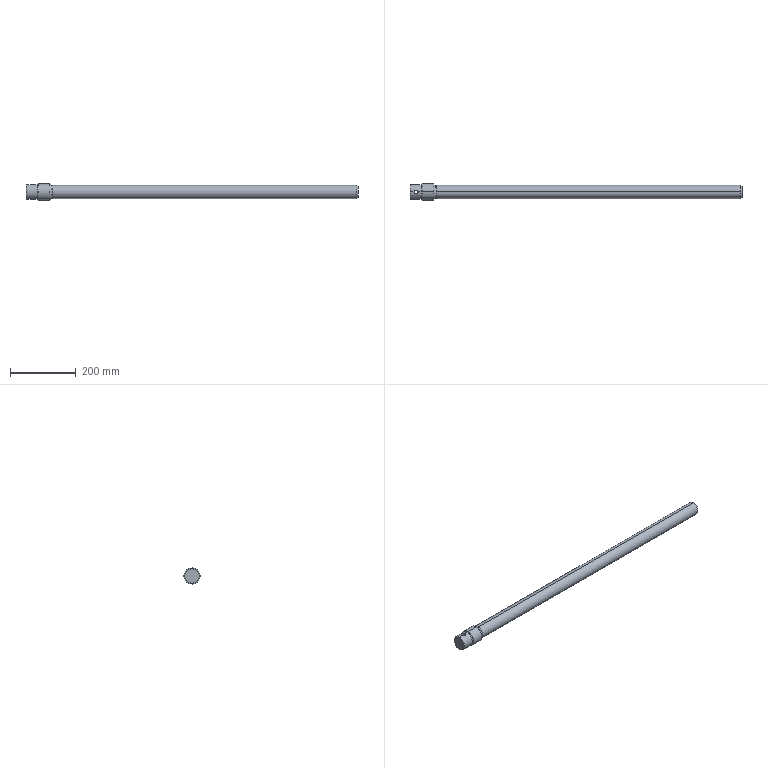Part | SolidWorks | features Chamfer 2, HoleWzd 1, ICE 1, Revolution 1 | 1 solid | 27 faces | box 1010 x 50 x 50 mm | volume 1298621 mm3 | cylinder 14 | cone 8 | plane 5 | commonest cylinder face diameters 10.2 x2 12 x2 39 x2 40 x2 40.6 x2 45 x2
STEP:
#1=CARTESIAN_POINT('',(986.75,0.,5.1));
#2=VERTEX_POINT('',#1);
#3=CARTESIAN_POINT('',(986.75,0.,-5.1));
#4=VERTEX_POINT('',#3);
#5=CARTESIAN_POINT('',(986.75,0.,0.));
#6=DIRECTION('',(1.,0.,0.));
#7=DIRECTION('',(0.,0.,-1.));
#8=AXIS2_PLACEMENT_3D('',#5,#6,#7);
#9=CIRCLE('',#8,5.1);
#10=EDGE_CURVE('',#2,#4,#9,.T.);
#11=ORIENTED_EDGE('',*,*,#10,.F.);
#12=CARTESIAN_POINT('',(1010.,0.,5.1));
#13=VERTEX_POINT('',#12);
#14=CARTESIAN_POINT('',(1010.,0.,5.1));
#15=DIRECTION('',(1.,0.,0.));
#16=VECTOR('',#15,1000.);
#17=LINE('',#14,#16);
#18=EDGE_CURVE('',#2,#13,#17,.T.);
#19=ORIENTED_EDGE('',*,*,#18,.T.);
#20=CARTESIAN_POINT('',(1010.,0.,-5.1));
#21=VERTEX_POINT('',#20);
#22=CARTESIAN_POINT('',(1010.,0.,0.));
#23=DIRECTION('',(1.,0.,0.));
#24=DIRECTION('',(0.,0.,-1.));
#25=AXIS2_PLACEMENT_3D('',#22,#23,#24);
#26=CIRCLE('',#25,5.1);
#27=EDGE_CURVE('',#13,#21,#26,.T.);
#28=ORIENTED_EDGE('',*,*,#27,.T.);
#29=CARTESIAN_POINT('',(1010.,0.,-5.1));
#30=DIRECTION('',(1.,0.,0.));
#31=VECTOR('',#30,1000.);
#32=LINE('',#29,#31);
#33=EDGE_CURVE('',#4,#21,#32,.T.);
#34=ORIENTED_EDGE('',*,*,#33,.F.);
#35=EDGE_LOOP('',(#11,#19,#28,#34));
#36=FACE_OUTER_BOUND('',#35,.T.);
#37=CARTESIAN_POINT('',(1010.,0.,0.));
#38=DIRECTION('',(1.,0.,0.));
#39=DIRECTION('',(0.,0.,-1.));
#40=AXIS2_PLACEMENT_3D('',#37,#38,#39);
#41=CYLINDRICAL_SURFACE('',#40,5.1);
#42=ADVANCED_FACE('',(#36),#41,.F.);
#43=CARTESIAN_POINT('',(983.686,0.,0.));
#44=VERTEX_POINT('',#43);
#45=CARTESIAN_POINT('',(986.75,0.,-5.1));
#46=DIRECTION('',(0.515,0.,-0.8572));
#47=VECTOR('',#46,1000.);
#48=LINE('',#45,#47);
#49=EDGE_CURVE('',#44,#4,#48,.T.);
#50=ORIENTED_EDGE('',*,*,#49,.F.);
#51=CARTESIAN_POINT('',(986.75,0.,5.1));
#52=DIRECTION('',(0.515,0.,0.8572));
#53=VECTOR('',#52,1000.);
#54=LINE('',#51,#53);
#55=EDGE_CURVE('',#44,#2,#54,.T.);
#56=ORIENTED_EDGE('',*,*,#55,.T.);
#57=ORIENTED_EDGE('',*,*,#10,.T.);
#58=EDGE_LOOP('',(#50,#56,#57));
#59=FACE_OUTER_BOUND('',#58,.T.);
#60=CARTESIAN_POINT('',(986.75,0.,0.));
#61=DIRECTION('',(1.,0.,0.));
#62=DIRECTION('',(0.,0.,-1.));
#63=AXIS2_PLACEMENT_3D('',#60,#61,#62);
#64=CONICAL_SURFACE('',#63,5.1,1.03);
#65=ADVANCED_FACE('',(#59),#64,.F.);
#66=CARTESIAN_POINT('',(24.5,0.,-22.5));
#67=VERTEX_POINT('',#66);
#68=CARTESIAN_POINT('',(12.5,0.,-22.5));
#69=VERTEX_POINT('',#68);
#70=CARTESIAN_POINT('',(24.5,0.,-22.5));
#71=CARTESIAN_POINT('',(24.5,-0.3984,-22.5));
#72=CARTESIAN_POINT('',(24.461,-0.7897,-22.489));
#73=CARTESIAN_POINT('',(24.346,-1.367,-22.459));
#74=CARTESIAN_POINT('',(24.298,-1.557,-22.447));
#75=CARTESIAN_POINT('',(24.183,-1.935,-22.417));
#76=CARTESIAN_POINT('',(24.115,-2.123,-22.4));
#77=CARTESIAN_POINT('',(23.889,-2.667,-22.344));
#78=CARTESIAN_POINT('',(23.704,-3.011,-22.3));
#79=CARTESIAN_POINT('',(23.378,-3.499,-22.227));
#80=CARTESIAN_POINT('',(23.26,-3.658,-22.201));
#81=CARTESIAN_POINT('',(23.01,-3.962,-22.149));
#82=CARTESIAN_POINT('',(22.879,-4.106,-22.123));
#83=CARTESIAN_POINT('',(22.466,-4.519,-22.043));
#84=CARTESIAN_POINT('',(22.165,-4.767,-21.99));
#85=CARTESIAN_POINT('',(21.51,-5.206,-21.891));
#86=CARTESIAN_POINT('',(21.163,-5.391,-21.845));
#87=CARTESIAN_POINT('',(20.622,-5.616,-21.788));
#88=CARTESIAN_POINT('',(20.438,-5.682,-21.771));
#89=CARTESIAN_POINT('',(20.062,-5.797,-21.741));
#90=CARTESIAN_POINT('',(19.868,-5.845,-21.727));
#91=CARTESIAN_POINT('',(19.286,-5.961,-21.696));
#92=CARTESIAN_POINT('',(18.896,-6.,-21.685));
#93=CARTESIAN_POINT('',(18.109,-6.,-21.685));
#94=CARTESIAN_POINT('',(17.71,-5.961,-21.696));
#95=CARTESIAN_POINT('',(16.939,-5.807,-21.738));
#96=CARTESIAN_POINT('',(16.564,-5.693,-21.769));
#97=CARTESIAN_POINT('',(16.017,-5.466,-21.826));
#98=CARTESIAN_POINT('',(15.838,-5.381,-21.847));
#99=CARTESIAN_POINT('',(15.492,-5.195,-21.892));
#100=CARTESIAN_POINT('',(15.325,-5.095,-21.916));
#101=CARTESIAN_POINT('',(15.001,-4.878,-21.965));
#102=CARTESIAN_POINT('',(14.844,-4.762,-21.991));
#103=CARTESIAN_POINT('',(14.542,-4.513,-22.043));
#104=CARTESIAN_POINT('',(14.395,-4.38,-22.07));
#105=CARTESIAN_POINT('',(13.979,-3.964,-22.15));
#106=CARTESIAN_POINT('',(13.732,-3.663,-22.202));
#107=CARTESIAN_POINT('',(13.297,-3.014,-22.3));
#108=CARTESIAN_POINT('',(13.109,-2.663,-22.345));
#109=CARTESIAN_POINT('',(12.808,-1.939,-22.419));
#110=CARTESIAN_POINT('',(12.694,-1.565,-22.449));
#111=CARTESIAN_POINT('',(12.578,-0.9844,-22.479));
#112=CARTESIAN_POINT('',(12.549,-0.7867,-22.487));
#113=CARTESIAN_POINT('',(12.51,-0.3929,-22.497));
#114=CARTESIAN_POINT('',(12.5,-0.1963,-22.5));
#115=CARTESIAN_POINT('',(12.5,0.,-22.5));
#116=B_SPLINE_CURVE_WITH_KNOTS('',3,(#70,#71,#72,#73,#74,#75,#76,#77,#78,#79,#80,#81,#82,#83,#84,#85,#86,#87,#88,#89,#90,#91,#92,#93,#94,#95,#96,#97,#98,#99,#100,#101,#102,#103,#104,#105,#106,#107,#108,#109,#110,#111,#112,#113,#114,#115),.UNSPECIFIED.,.F.,.F.,(4,2,2,2,2,2,2,2,2,2,2,2,2,2,2,2,2,2,2,2,2,2,4),(0.,0.001178,0.001767,0.002356,0.003533,0.004122,0.004711,0.005889,0.007067,0.007656,0.008244,0.009422,0.0106,0.01178,0.01237,0.01296,0.01354,0.01413,0.01531,0.01649,0.01767,0.01826,0.01884),.UNSPECIFIED.);
#117=EDGE_CURVE('',#67,#69,#116,.T.);
#118=ORIENTED_EDGE('',*,*,#117,.T.);
#119=CARTESIAN_POINT('',(12.5,0.,22.5));
#120=VERTEX_POINT('',#119);
#121=CARTESIAN_POINT('',(12.5,0.,-50.));
#122=DIRECTION('',(0.,0.,1.));
#123=VECTOR('',#122,1000.);
#124=LINE('',#121,#123);
#125=EDGE_CURVE('',#69,#120,#124,.T.);
#126=ORIENTED_EDGE('',*,*,#125,.T.);
#127=CARTESIAN_POINT('',(24.5,0.,22.5));
#128=VERTEX_POINT('',#127);
#129=CARTESIAN_POINT('',(12.5,0.,22.5));
#130=CARTESIAN_POINT('',(12.5,-0.3926,22.5));
#131=CARTESIAN_POINT('',(12.538,-0.7847,22.49));
#132=CARTESIAN_POINT('',(12.694,-1.564,22.449));
#133=CARTESIAN_POINT('',(12.809,-1.939,22.419));
#134=CARTESIAN_POINT('',(13.109,-2.662,22.345));
#135=CARTESIAN_POINT('',(13.297,-3.013,22.3));
#136=CARTESIAN_POINT('',(13.732,-3.664,22.202));
#137=CARTESIAN_POINT('',(13.979,-3.965,22.15));
#138=CARTESIAN_POINT('',(14.394,-4.38,22.07));
#139=CARTESIAN_POINT('',(14.541,-4.513,22.043));
#140=CARTESIAN_POINT('',(14.844,-4.762,21.991));
#141=CARTESIAN_POINT('',(15.001,-4.878,21.965));
#142=CARTESIAN_POINT('',(15.487,-5.203,21.891));
#143=CARTESIAN_POINT('',(15.83,-5.388,21.846));
#144=CARTESIAN_POINT('',(16.561,-5.692,21.769));
#145=CARTESIAN_POINT('',(16.938,-5.806,21.738));
#146=CARTESIAN_POINT('',(17.514,-5.922,21.707));
#147=CARTESIAN_POINT('',(17.708,-5.951,21.699));
#148=CARTESIAN_POINT('',(18.101,-5.99,21.688));
#149=CARTESIAN_POINT('',(18.301,-6.,21.685));
#150=CARTESIAN_POINT('',(18.894,-6.,21.685));
#151=CARTESIAN_POINT('',(19.285,-5.961,21.696));
#152=CARTESIAN_POINT('',(20.056,-5.808,21.738));
#153=CARTESIAN_POINT('',(20.439,-5.692,21.769));
#154=CARTESIAN_POINT('',(21.162,-5.391,21.845));
#155=CARTESIAN_POINT('',(21.507,-5.207,21.89));
#156=CARTESIAN_POINT('',(22.162,-4.769,21.99));
#157=CARTESIAN_POINT('',(22.465,-4.52,22.043));
#158=CARTESIAN_POINT('',(22.878,-4.107,22.122));
#159=CARTESIAN_POINT('',(23.009,-3.963,22.149));
#160=CARTESIAN_POINT('',(23.258,-3.661,22.201));
#161=CARTESIAN_POINT('',(23.376,-3.502,22.226));
#162=CARTESIAN_POINT('',(23.704,-3.012,22.3));
#163=CARTESIAN_POINT('',(23.888,-2.668,22.344));
#164=CARTESIAN_POINT('',(24.189,-1.946,22.419));
#165=CARTESIAN_POINT('',(24.306,-1.563,22.449));
#166=CARTESIAN_POINT('',(24.461,-0.7906,22.489));
#167=CARTESIAN_POINT('',(24.5,-0.3983,22.5));
#168=CARTESIAN_POINT('',(24.5,0.,22.5));
#169=B_SPLINE_CURVE_WITH_KNOTS('',3,(#129,#130,#131,#132,#133,#134,#135,#136,#137,#138,#139,#140,#141,#142,#143,#144,#145,#146,#147,#148,#149,#150,#151,#152,#153,#154,#155,#156,#157,#158,#159,#160,#161,#162,#163,#164,#165,#166,#167,#168),.UNSPECIFIED.,.F.,.F.,(4,2,2,2,2,2,2,2,2,2,2,2,2,2,2,2,2,2,2,4),(0.01884,0.02002,0.0212,0.02238,0.02355,0.02414,0.02473,0.02591,0.02709,0.02768,0.02826,0.02944,0.03062,0.0318,0.03297,0.03356,0.03415,0.03533,0.03651,0.03768),.UNSPECIFIED.);
#170=EDGE_CURVE('',#120,#128,#169,.T.);
#171=ORIENTED_EDGE('',*,*,#170,.T.);
#172=CARTESIAN_POINT('',(24.5,0.,-50.));
#173=DIRECTION('',(0.,0.,1.));
#174=VECTOR('',#173,1000.);
#175=LINE('',#172,#174);
#176=EDGE_CURVE('',#67,#128,#175,.T.);
#177=ORIENTED_EDGE('',*,*,#176,.F.);
#178=EDGE_LOOP('',(#118,#126,#171,#177));
#179=FACE_OUTER_BOUND('',#178,.T.);
#180=CARTESIAN_POINT('',(18.5,0.,-50.));
#181=DIRECTION('',(0.,0.,1.));
#182=DIRECTION('',(1.,0.,0.));
#183=AXIS2_PLACEMENT_3D('',#180,#181,#182);
#184=CYLINDRICAL_SURFACE('',#183,6.);
#185=ADVANCED_FACE('',(#179),#184,.F.);
#186=CARTESIAN_POINT('',(0.,0.,21.5));
#187=VERTEX_POINT('',#186);
#188=CARTESIAN_POINT('',(0.,0.,-21.5));
#189=VERTEX_POINT('',#188);
#190=CARTESIAN_POINT('',(0.,0.,0.));
#191=DIRECTION('',(-1.,0.,0.));
#192=DIRECTION('',(0.,0.,1.));
#193=AXIS2_PLACEMENT_3D('',#190,#191,#192);
#194=CIRCLE('',#193,21.5);
#195=EDGE_CURVE('',#187,#189,#194,.T.);
#196=ORIENTED_EDGE('',*,*,#195,.F.);
#197=CARTESIAN_POINT('',(1.,0.,22.5));
#198=VERTEX_POINT('',#197);
#199=CARTESIAN_POINT('',(0.,0.,21.5));
#200=DIRECTION('',(0.7071,0.,0.7071));
#201=VECTOR('',#200,1000.);
#202=LINE('',#199,#201);
#203=EDGE_CURVE('',#187,#198,#202,.T.);
#204=ORIENTED_EDGE('',*,*,#203,.T.);
#205=CARTESIAN_POINT('',(1.,0.,-22.5));
#206=VERTEX_POINT('',#205);
#207=CARTESIAN_POINT('',(1.,0.,0.));
#208=DIRECTION('',(1.,0.,0.));
#209=DIRECTION('',(0.,0.,1.));
#210=AXIS2_PLACEMENT_3D('',#207,#208,#209);
#211=CIRCLE('',#210,22.5);
#212=EDGE_CURVE('',#206,#198,#211,.T.);
#213=ORIENTED_EDGE('',*,*,#212,.F.);
#214=CARTESIAN_POINT('',(0.,0.,-21.5));
#215=DIRECTION('',(0.7071,0.,-0.7071));
#216=VECTOR('',#215,1000.);
#217=LINE('',#214,#216);
#218=EDGE_CURVE('',#189,#206,#217,.T.);
#219=ORIENTED_EDGE('',*,*,#218,.F.);
#220=EDGE_LOOP('',(#196,#204,#213,#219));
#221=FACE_OUTER_BOUND('',#220,.T.);
#222=CARTESIAN_POINT('',(0.,0.,0.));
#223=DIRECTION('',(1.,0.,0.));
#224=DIRECTION('',(0.,0.,-1.));
#225=AXIS2_PLACEMENT_3D('',#222,#223,#224);
#226=CONICAL_SURFACE('',#225,21.5,0.7854);
#227=ADVANCED_FACE('',(#221),#226,.T.);
#228=CARTESIAN_POINT('',(1010.,0.,-16.5));
#229=VERTEX_POINT('',#228);
#230=CARTESIAN_POINT('',(1010.,0.,16.5));
#231=VERTEX_POINT('',#230);
#232=CARTESIAN_POINT('',(1010.,0.,0.));
#233=DIRECTION('',(1.,0.,0.));
#234=DIRECTION('',(0.,0.,1.));
#235=AXIS2_PLACEMENT_3D('',#232,#233,#234);
#236=CIRCLE('',#235,16.5);
#237=EDGE_CURVE('',#229,#231,#236,.T.);
#238=ORIENTED_EDGE('',*,*,#237,.F.);
#239=CARTESIAN_POINT('',(1006.5,0.,-20.));
#240=VERTEX_POINT('',#239);
#241=CARTESIAN_POINT('',(1006.5,0.,-20.));
#242=DIRECTION('',(-0.7071,0.,-0.7071));
#243=VECTOR('',#242,1000.);
#244=LINE('',#241,#243);
#245=EDGE_CURVE('',#229,#240,#244,.T.);
#246=ORIENTED_EDGE('',*,*,#245,.T.);
#247=CARTESIAN_POINT('',(1006.5,0.,20.));
#248=VERTEX_POINT('',#247);
#249=CARTESIAN_POINT('',(1006.5,0.,0.));
#250=DIRECTION('',(-1.,0.,0.));
#251=DIRECTION('',(0.,0.,1.));
#252=AXIS2_PLACEMENT_3D('',#249,#250,#251);
#253=CIRCLE('',#252,20.);
#254=EDGE_CURVE('',#248,#240,#253,.T.);
#255=ORIENTED_EDGE('',*,*,#254,.F.);
#256=CARTESIAN_POINT('',(1006.5,0.,20.));
#257=DIRECTION('',(-0.7071,0.,0.7071));
#258=VECTOR('',#257,1000.);
#259=LINE('',#256,#258);
#260=EDGE_CURVE('',#231,#248,#259,.T.);
#261=ORIENTED_EDGE('',*,*,#260,.F.);
#262=EDGE_LOOP('',(#238,#246,#255,#261));
#263=FACE_OUTER_BOUND('',#262,.T.);
#264=CARTESIAN_POINT('',(1006.5,0.,0.));
#265=DIRECTION('',(-1.,0.,0.));
#266=DIRECTION('',(0.,0.,1.));
#267=AXIS2_PLACEMENT_3D('',#264,#265,#266);
#268=CONICAL_SURFACE('',#267,20.,0.7854);
#269=ADVANCED_FACE('',(#263),#268,.T.);
#270=CARTESIAN_POINT('',(38.,0.,20.3));
#271=VERTEX_POINT('',#270);
#272=CARTESIAN_POINT('',(38.,0.,-20.3));
#273=VERTEX_POINT('',#272);
#274=CARTESIAN_POINT('',(38.,0.,0.));
#275=DIRECTION('',(-1.,0.,0.));
#276=DIRECTION('',(0.,0.,1.));
#277=AXIS2_PLACEMENT_3D('',#274,#275,#276);
#278=CIRCLE('',#277,20.3);
#279=EDGE_CURVE('',#271,#273,#278,.T.);
#280=ORIENTED_EDGE('',*,*,#279,.T.);
#281=CARTESIAN_POINT('',(33.5,0.,-20.3));
#282=VERTEX_POINT('',#281);
#283=CARTESIAN_POINT('',(38.,0.,-20.3));
#284=DIRECTION('',(-1.,0.,0.));
#285=VECTOR('',#284,1000.);
#286=LINE('',#283,#285);
#287=EDGE_CURVE('',#273,#282,#286,.T.);
#288=ORIENTED_EDGE('',*,*,#287,.T.);
#289=CARTESIAN_POINT('',(33.5,0.,20.3));
#290=VERTEX_POINT('',#289);
#291=CARTESIAN_POINT('',(33.5,0.,0.));
#292=DIRECTION('',(-1.,0.,0.));
#293=DIRECTION('',(0.,0.,1.));
#294=AXIS2_PLACEMENT_3D('',#291,#292,#293);
#295=CIRCLE('',#294,20.3);
#296=EDGE_CURVE('',#290,#282,#295,.T.);
#297=ORIENTED_EDGE('',*,*,#296,.F.);
#298=CARTESIAN_POINT('',(38.,0.,20.3));
#299=DIRECTION('',(-1.,0.,0.));
#300=VECTOR('',#299,1000.);
#301=LINE('',#298,#300);
#302=EDGE_CURVE('',#271,#290,#301,.T.);
#303=ORIENTED_EDGE('',*,*,#302,.F.);
#304=EDGE_LOOP('',(#280,#288,#297,#303));
#305=FACE_OUTER_BOUND('',#304,.T.);
#306=CARTESIAN_POINT('',(38.,0.,0.));
#307=DIRECTION('',(-1.,0.,0.));
#308=DIRECTION('',(0.,0.,1.));
#309=AXIS2_PLACEMENT_3D('',#306,#307,#308);
#310=CYLINDRICAL_SURFACE('',#309,20.3);
#311=ADVANCED_FACE('',(#305),#310,.T.);
#312=CARTESIAN_POINT('',(72.5,0.,25.));
#313=VERTEX_POINT('',#312);
#314=CARTESIAN_POINT('',(72.5,0.,-25.));
#315=VERTEX_POINT('',#314);
#316=CARTESIAN_POINT('',(72.5,0.,0.));
#317=DIRECTION('',(-1.,0.,0.));
#318=DIRECTION('',(0.,0.,1.));
#319=AXIS2_PLACEMENT_3D('',#316,#317,#318);
#320=CIRCLE('',#319,25.);
#321=EDGE_CURVE('',#313,#315,#320,.T.);
#322=ORIENTED_EDGE('',*,*,#321,.T.);
#323=CARTESIAN_POINT('',(38.,0.,-25.));
#324=VERTEX_POINT('',#323);
#325=CARTESIAN_POINT('',(38.,0.,-25.));
#326=DIRECTION('',(-1.,0.,0.));
#327=VECTOR('',#326,1000.);
#328=LINE('',#325,#327);
#329=EDGE_CURVE('',#315,#324,#328,.T.);
#330=ORIENTED_EDGE('',*,*,#329,.T.);
#331=CARTESIAN_POINT('',(38.,0.,25.));
#332=VERTEX_POINT('',#331);
#333=CARTESIAN_POINT('',(38.,0.,0.));
#334=DIRECTION('',(-1.,0.,0.));
#335=DIRECTION('',(0.,0.,1.));
#336=AXIS2_PLACEMENT_3D('',#333,#334,#335);
#337=CIRCLE('',#336,25.);
#338=EDGE_CURVE('',#332,#324,#337,.T.);
#339=ORIENTED_EDGE('',*,*,#338,.F.);
#340=CARTESIAN_POINT('',(38.,0.,25.));
#341=DIRECTION('',(-1.,0.,0.));
#342=VECTOR('',#341,1000.);
#343=LINE('',#340,#342);
#344=EDGE_CURVE('',#313,#332,#343,.T.);
#345=ORIENTED_EDGE('',*,*,#344,.F.);
#346=EDGE_LOOP('',(#322,#330,#339,#345));
#347=FACE_OUTER_BOUND('',#346,.T.);
#348=CARTESIAN_POINT('',(38.,0.,0.));
#349=DIRECTION('',(-1.,0.,0.));
#350=DIRECTION('',(0.,0.,1.));
#351=AXIS2_PLACEMENT_3D('',#348,#349,#350);
#352=CYLINDRICAL_SURFACE('',#351,25.);
#353=ADVANCED_FACE('',(#347),#352,.T.);
#354=CARTESIAN_POINT('',(78.,0.,19.5));
#355=VERTEX_POINT('',#354);
#356=CARTESIAN_POINT('',(78.,0.,-19.5));
#357=VERTEX_POINT('',#356);
#358=CARTESIAN_POINT('',(78.,0.,0.));
#359=DIRECTION('',(-1.,0.,0.));
#360=DIRECTION('',(0.,0.,1.));
#361=AXIS2_PLACEMENT_3D('',#358,#359,#360);
#362=CIRCLE('',#361,19.5);
#363=EDGE_CURVE('',#355,#357,#362,.T.);
#364=ORIENTED_EDGE('',*,*,#363,.T.);
#365=CARTESIAN_POINT('',(78.,0.,-19.5));
#366=DIRECTION('',(-0.7071,0.,-0.7071));
#367=VECTOR('',#366,1000.);
#368=LINE('',#365,#367);
#369=EDGE_CURVE('',#357,#315,#368,.T.);
#370=ORIENTED_EDGE('',*,*,#369,.T.);
#371=ORIENTED_EDGE('',*,*,#321,.F.);
#372=CARTESIAN_POINT('',(78.,0.,19.5));
#373=DIRECTION('',(-0.7071,0.,0.7071));
#374=VECTOR('',#373,1000.);
#375=LINE('',#372,#374);
#376=EDGE_CURVE('',#355,#313,#375,.T.);
#377=ORIENTED_EDGE('',*,*,#376,.F.);
#378=EDGE_LOOP('',(#364,#370,#371,#377));
#379=FACE_OUTER_BOUND('',#378,.T.);
#380=CARTESIAN_POINT('',(78.,0.,0.));
#381=DIRECTION('',(-1.,0.,0.));
#382=DIRECTION('',(0.,0.,1.));
#383=AXIS2_PLACEMENT_3D('',#380,#381,#382);
#384=CONICAL_SURFACE('',#383,19.5,0.7854);
#385=ADVANCED_FACE('',(#379),#384,.T.);
#386=CARTESIAN_POINT('',(81.,0.,19.5));
#387=VERTEX_POINT('',#386);
#388=CARTESIAN_POINT('',(81.,0.,-19.5));
#389=VERTEX_POINT('',#388);
#390=CARTESIAN_POINT('',(81.,0.,0.));
#391=DIRECTION('',(-1.,0.,0.));
#392=DIRECTION('',(0.,0.,1.));
#393=AXIS2_PLACEMENT_3D('',#390,#391,#392);
#394=CIRCLE('',#393,19.5);
#395=EDGE_CURVE('',#387,#389,#394,.T.);
#396=ORIENTED_EDGE('',*,*,#395,.T.);
#397=CARTESIAN_POINT('',(38.,0.,-19.5));
#398=DIRECTION('',(-1.,0.,0.));
#399=VECTOR('',#398,1000.);
#400=LINE('',#397,#399);
#401=EDGE_CURVE('',#389,#357,#400,.T.);
#402=ORIENTED_EDGE('',*,*,#401,.T.);
#403=ORIENTED_EDGE('',*,*,#363,.F.);
#404=CARTESIAN_POINT('',(38.,0.,19.5));
#405=DIRECTION('',(-1.,0.,0.));
#406=VECTOR('',#405,1000.);
#407=LINE('',#404,#406);
#408=EDGE_CURVE('',#387,#355,#407,.T.);
#409=ORIENTED_EDGE('',*,*,#408,.F.);
#410=EDGE_LOOP('',(#396,#402,#403,#409));
#411=FACE_OUTER_BOUND('',#410,.T.);
#412=CARTESIAN_POINT('',(38.,0.,0.));
#413=DIRECTION('',(-1.,0.,0.));
#414=DIRECTION('',(0.,0.,1.));
#415=AXIS2_PLACEMENT_3D('',#412,#413,#414);
#416=CYLINDRICAL_SURFACE('',#415,19.5);
#417=ADVANCED_FACE('',(#411),#416,.T.);
#418=ORIENTED_EDGE('',*,*,#254,.T.);
#419=CARTESIAN_POINT('',(81.,0.,-20.));
#420=VERTEX_POINT('',#419);
#421=CARTESIAN_POINT('',(38.,0.,-20.));
#422=DIRECTION('',(-1.,0.,0.));
#423=VECTOR('',#422,1000.);
#424=LINE('',#421,#423);
#425=EDGE_CURVE('',#240,#420,#424,.T.);
#426=ORIENTED_EDGE('',*,*,#425,.T.);
#427=CARTESIAN_POINT('',(81.,0.,20.));
#428=VERTEX_POINT('',#427);
#429=CARTESIAN_POINT('',(81.,0.,0.));
#430=DIRECTION('',(-1.,0.,0.));
#431=DIRECTION('',(0.,0.,1.));
#432=AXIS2_PLACEMENT_3D('',#429,#430,#431);
#433=CIRCLE('',#432,20.);
#434=EDGE_CURVE('',#428,#420,#433,.T.);
#435=ORIENTED_EDGE('',*,*,#434,.F.);
#436=CARTESIAN_POINT('',(38.,0.,20.));
#437=DIRECTION('',(-1.,0.,0.));
#438=VECTOR('',#437,1000.);
#439=LINE('',#436,#438);
#440=EDGE_CURVE('',#248,#428,#439,.T.);
#441=ORIENTED_EDGE('',*,*,#440,.F.);
#442=EDGE_LOOP('',(#418,#426,#435,#441));
#443=FACE_OUTER_BOUND('',#442,.T.);
#444=CARTESIAN_POINT('',(38.,0.,0.));
#445=DIRECTION('',(-1.,0.,0.));
#446=DIRECTION('',(0.,0.,1.));
#447=AXIS2_PLACEMENT_3D('',#444,#445,#446);
#448=CYLINDRICAL_SURFACE('',#447,20.);
#449=ADVANCED_FACE('',(#443),#448,.T.);
#450=CARTESIAN_POINT('',(33.5,0.,22.5));
#451=VERTEX_POINT('',#450);
#452=CARTESIAN_POINT('',(33.5,0.,-22.5));
#453=VERTEX_POINT('',#452);
#454=CARTESIAN_POINT('',(33.5,0.,0.));
#455=DIRECTION('',(-1.,0.,0.));
#456=DIRECTION('',(0.,0.,1.));
#457=AXIS2_PLACEMENT_3D('',#454,#455,#456);
#458=CIRCLE('',#457,22.5);
#459=EDGE_CURVE('',#451,#453,#458,.T.);
#460=ORIENTED_EDGE('',*,*,#459,.T.);
#461=CARTESIAN_POINT('',(38.,0.,-22.5));
#462=DIRECTION('',(-1.,0.,0.));
#463=VECTOR('',#462,1000.);
#464=LINE('',#461,#463);
#465=EDGE_CURVE('',#453,#67,#464,.T.);
#466=ORIENTED_EDGE('',*,*,#465,.T.);
#467=CARTESIAN_POINT('',(12.5,0.,-22.5));
#468=CARTESIAN_POINT('',(12.5,0.3926,-22.5));
#469=CARTESIAN_POINT('',(12.538,0.7847,-22.49));
#470=CARTESIAN_POINT('',(12.694,1.564,-22.449));
#471=CARTESIAN_POINT('',(12.809,1.939,-22.419));
#472=CARTESIAN_POINT('',(13.109,2.662,-22.345));
#473=CARTESIAN_POINT('',(13.297,3.013,-22.3));
#474=CARTESIAN_POINT('',(13.732,3.664,-22.202));
#475=CARTESIAN_POINT('',(13.979,3.965,-22.15));
#476=CARTESIAN_POINT('',(14.394,4.38,-22.07));
#477=CARTESIAN_POINT('',(14.541,4.513,-22.043));
#478=CARTESIAN_POINT('',(14.844,4.762,-21.991));
#479=CARTESIAN_POINT('',(15.001,4.878,-21.965));
#480=CARTESIAN_POINT('',(15.487,5.203,-21.891));
#481=CARTESIAN_POINT('',(15.83,5.388,-21.846));
#482=CARTESIAN_POINT('',(16.561,5.692,-21.769));
#483=CARTESIAN_POINT('',(16.938,5.806,-21.738));
#484=CARTESIAN_POINT('',(17.514,5.922,-21.707));
#485=CARTESIAN_POINT('',(17.708,5.951,-21.699));
#486=CARTESIAN_POINT('',(18.101,5.99,-21.688));
#487=CARTESIAN_POINT('',(18.301,6.,-21.685));
#488=CARTESIAN_POINT('',(18.894,6.,-21.685));
#489=CARTESIAN_POINT('',(19.285,5.961,-21.696));
#490=CARTESIAN_POINT('',(20.056,5.808,-21.738));
#491=CARTESIAN_POINT('',(20.439,5.692,-21.769));
#492=CARTESIAN_POINT('',(21.162,5.391,-21.845));
#493=CARTESIAN_POINT('',(21.507,5.207,-21.89));
#494=CARTESIAN_POINT('',(22.162,4.769,-21.99));
#495=CARTESIAN_POINT('',(22.465,4.52,-22.043));
#496=CARTESIAN_POINT('',(22.878,4.107,-22.122));
#497=CARTESIAN_POINT('',(23.009,3.963,-22.149));
#498=CARTESIAN_POINT('',(23.258,3.661,-22.201));
#499=CARTESIAN_POINT('',(23.376,3.502,-22.226));
#500=CARTESIAN_POINT('',(23.704,3.012,-22.3));
#501=CARTESIAN_POINT('',(23.888,2.668,-22.344));
#502=CARTESIAN_POINT('',(24.189,1.946,-22.419));
#503=CARTESIAN_POINT('',(24.306,1.563,-22.449));
#504=CARTESIAN_POINT('',(24.461,0.7906,-22.489));
#505=CARTESIAN_POINT('',(24.5,0.3983,-22.5));
#506=CARTESIAN_POINT('',(24.5,0.,-22.5));
#507=B_SPLINE_CURVE_WITH_KNOTS('',3,(#467,#468,#469,#470,#471,#472,#473,#474,#475,#476,#477,#478,#479,#480,#481,#482,#483,#484,#485,#486,#487,#488,#489,#490,#491,#492,#493,#494,#495,#496,#497,#498,#499,#500,#501,#502,#503,#504,#505,#506),.UNSPECIFIED.,.F.,.F.,(4,2,2,2,2,2,2,2,2,2,2,2,2,2,2,2,2,2,2,4),(0.01884,0.02002,0.0212,0.02238,0.02355,0.02414,0.02473,0.02591,0.02709,0.02768,0.02826,0.02944,0.03062,0.0318,0.03297,0.03356,0.03415,0.03533,0.03651,0.03768),.UNSPECIFIED.);
#508=EDGE_CURVE('',#69,#67,#507,.T.);
#509=ORIENTED_EDGE('',*,*,#508,.F.);
#510=CARTESIAN_POINT('',(38.,0.,-22.5));
#511=DIRECTION('',(-1.,0.,0.));
#512=VECTOR('',#511,1000.);
#513=LINE('',#510,#512);
#514=EDGE_CURVE('',#69,#206,#513,.T.);
#515=ORIENTED_EDGE('',*,*,#514,.T.);
#516=ORIENTED_EDGE('',*,*,#212,.T.);
#517=CARTESIAN_POINT('',(38.,0.,22.5));
#518=DIRECTION('',(-1.,0.,0.));
#519=VECTOR('',#518,1000.);
#520=LINE('',#517,#519);
#521=EDGE_CURVE('',#120,#198,#520,.T.);
#522=ORIENTED_EDGE('',*,*,#521,.F.);
#523=CARTESIAN_POINT('',(24.5,0.,22.5));
#524=CARTESIAN_POINT('',(24.5,0.3984,22.5));
#525=CARTESIAN_POINT('',(24.461,0.7897,22.489));
#526=CARTESIAN_POINT('',(24.346,1.367,22.459));
#527=CARTESIAN_POINT('',(24.298,1.557,22.447));
#528=CARTESIAN_POINT('',(24.183,1.935,22.417));
#529=CARTESIAN_POINT('',(24.115,2.123,22.4));
#530=CARTESIAN_POINT('',(23.889,2.667,22.344));
#531=CARTESIAN_POINT('',(23.704,3.011,22.3));
#532=CARTESIAN_POINT('',(23.378,3.499,22.227));
#533=CARTESIAN_POINT('',(23.26,3.658,22.201));
#534=CARTESIAN_POINT('',(23.01,3.962,22.149));
#535=CARTESIAN_POINT('',(22.879,4.106,22.123));
#536=CARTESIAN_POINT('',(22.466,4.519,22.043));
#537=CARTESIAN_POINT('',(22.165,4.767,21.99));
#538=CARTESIAN_POINT('',(21.51,5.206,21.891));
#539=CARTESIAN_POINT('',(21.163,5.391,21.845));
#540=CARTESIAN_POINT('',(20.622,5.616,21.788));
#541=CARTESIAN_POINT('',(20.438,5.682,21.771));
#542=CARTESIAN_POINT('',(20.062,5.797,21.741));
#543=CARTESIAN_POINT('',(19.868,5.845,21.727));
#544=CARTESIAN_POINT('',(19.286,5.961,21.696));
#545=CARTESIAN_POINT('',(18.896,6.,21.685));
#546=CARTESIAN_POINT('',(18.109,6.,21.685));
#547=CARTESIAN_POINT('',(17.71,5.961,21.696));
#548=CARTESIAN_POINT('',(16.939,5.807,21.738));
#549=CARTESIAN_POINT('',(16.564,5.693,21.769));
#550=CARTESIAN_POINT('',(16.017,5.466,21.826));
#551=CARTESIAN_POINT('',(15.838,5.381,21.847));
#552=CARTESIAN_POINT('',(15.492,5.195,21.892));
#553=CARTESIAN_POINT('',(15.325,5.095,21.916));
#554=CARTESIAN_POINT('',(15.001,4.878,21.965));
#555=CARTESIAN_POINT('',(14.844,4.762,21.991));
#556=CARTESIAN_POINT('',(14.542,4.513,22.043));
#557=CARTESIAN_POINT('',(14.395,4.38,22.07));
#558=CARTESIAN_POINT('',(13.979,3.964,22.15));
#559=CARTESIAN_POINT('',(13.732,3.663,22.202));
#560=CARTESIAN_POINT('',(13.297,3.014,22.3));
#561=CARTESIAN_POINT('',(13.109,2.663,22.345));
#562=CARTESIAN_POINT('',(12.808,1.939,22.419));
#563=CARTESIAN_POINT('',(12.694,1.565,22.449));
#564=CARTESIAN_POINT('',(12.578,0.9844,22.479));
#565=CARTESIAN_POINT('',(12.549,0.7867,22.487));
#566=CARTESIAN_POINT('',(12.51,0.3929,22.497));
#567=CARTESIAN_POINT('',(12.5,0.1963,22.5));
#568=CARTESIAN_POINT('',(12.5,0.,22.5));
#569=B_SPLINE_CURVE_WITH_KNOTS('',3,(#523,#524,#525,#526,#527,#528,#529,#530,#531,#532,#533,#534,#535,#536,#537,#538,#539,#540,#541,#542,#543,#544,#545,#546,#547,#548,#549,#550,#551,#552,#553,#554,#555,#556,#557,#558,#559,#560,#561,#562,#563,#564,#565,#566,#567,#568),.UNSPECIFIED.,.F.,.F.,(4,2,2,2,2,2,2,2,2,2,2,2,2,2,2,2,2,2,2,2,2,2,4),(0.,0.001178,0.001767,0.002356,0.003533,0.004122,0.004711,0.005889,0.007067,0.007656,0.008244,0.009422,0.0106,0.01178,0.01237,0.01296,0.01354,0.01413,0.01531,0.01649,0.01767,0.01826,0.01884),.UNSPECIFIED.);
#570=EDGE_CURVE('',#128,#120,#569,.T.);
#571=ORIENTED_EDGE('',*,*,#570,.F.);
#572=CARTESIAN_POINT('',(38.,0.,22.5));
#573=DIRECTION('',(-1.,0.,0.));
#574=VECTOR('',#573,1000.);
#575=LINE('',#572,#574);
#576=EDGE_CURVE('',#451,#128,#575,.T.);
#577=ORIENTED_EDGE('',*,*,#576,.F.);
#578=EDGE_LOOP('',(#460,#466,#509,#515,#516,#522,#571,#577));
#579=FACE_OUTER_BOUND('',#578,.T.);
#580=CARTESIAN_POINT('',(38.,0.,0.));
#581=DIRECTION('',(-1.,0.,0.));
#582=DIRECTION('',(0.,0.,1.));
#583=AXIS2_PLACEMENT_3D('',#580,#581,#582);
#584=CYLINDRICAL_SURFACE('',#583,22.5);
#585=ADVANCED_FACE('',(#579),#584,.T.);
#586=ORIENTED_EDGE('',*,*,#296,.T.);
#587=CARTESIAN_POINT('',(33.5,0.,0.));
#588=DIRECTION('',(-1.,0.,0.));
#589=DIRECTION('',(0.,0.,1.));
#590=AXIS2_PLACEMENT_3D('',#587,#588,#589);
#591=CIRCLE('',#590,20.3);
#592=EDGE_CURVE('',#282,#290,#591,.T.);
#593=ORIENTED_EDGE('',*,*,#592,.T.);
#594=EDGE_LOOP('',(#586,#593));
#595=FACE_BOUND('',#594,.T.);
#596=ORIENTED_EDGE('',*,*,#459,.F.);
#597=CARTESIAN_POINT('',(33.5,0.,0.));
#598=DIRECTION('',(-1.,0.,0.));
#599=DIRECTION('',(0.,0.,1.));
#600=AXIS2_PLACEMENT_3D('',#597,#598,#599);
#601=CIRCLE('',#600,22.5);
#602=EDGE_CURVE('',#453,#451,#601,.T.);
#603=ORIENTED_EDGE('',*,*,#602,.F.);
#604=EDGE_LOOP('',(#596,#603));
#605=FACE_OUTER_BOUND('',#604,.T.);
#606=CARTESIAN_POINT('',(33.5,0.,0.));
#607=DIRECTION('',(1.,0.,0.));
#608=DIRECTION('',(0.,0.,-1.));
#609=AXIS2_PLACEMENT_3D('',#606,#607,#608);
#610=PLANE('',#609);
#611=ADVANCED_FACE('',(#595,#605),#610,.T.);
#612=ORIENTED_EDGE('',*,*,#465,.F.);
#613=ORIENTED_EDGE('',*,*,#602,.T.);
#614=ORIENTED_EDGE('',*,*,#576,.T.);
#615=ORIENTED_EDGE('',*,*,#170,.F.);
#616=ORIENTED_EDGE('',*,*,#521,.T.);
#617=CARTESIAN_POINT('',(1.,0.,0.));
#618=DIRECTION('',(1.,0.,0.));
#619=DIRECTION('',(0.,0.,1.));
#620=AXIS2_PLACEMENT_3D('',#617,#618,#619);
#621=CIRCLE('',#620,22.5);
#622=EDGE_CURVE('',#198,#206,#621,.T.);
#623=ORIENTED_EDGE('',*,*,#622,.T.);
#624=ORIENTED_EDGE('',*,*,#514,.F.);
#625=ORIENTED_EDGE('',*,*,#117,.F.);
#626=EDGE_LOOP('',(#612,#613,#614,#615,#616,#623,#624,#625));
#627=FACE_OUTER_BOUND('',#626,.T.);
#628=CARTESIAN_POINT('',(38.,0.,0.));
#629=DIRECTION('',(-1.,0.,0.));
#630=DIRECTION('',(0.,0.,1.));
#631=AXIS2_PLACEMENT_3D('',#628,#629,#630);
#632=CYLINDRICAL_SURFACE('',#631,22.5);
#633=ADVANCED_FACE('',(#627),#632,.T.);
#634=CARTESIAN_POINT('',(0.,0.,0.));
#635=DIRECTION('',(-1.,0.,0.));
#636=DIRECTION('',(0.,0.,1.));
#637=AXIS2_PLACEMENT_3D('',#634,#635,#636);
#638=CIRCLE('',#637,21.5);
#639=EDGE_CURVE('',#189,#187,#638,.T.);
#640=ORIENTED_EDGE('',*,*,#639,.T.);
#641=ORIENTED_EDGE('',*,*,#195,.T.);
#642=EDGE_LOOP('',(#640,#641));
#643=FACE_OUTER_BOUND('',#642,.T.);
#644=CARTESIAN_POINT('',(0.,0.,0.));
#645=DIRECTION('',(-1.,0.,0.));
#646=DIRECTION('',(0.,0.,1.));
#647=AXIS2_PLACEMENT_3D('',#644,#645,#646);
#648=PLANE('',#647);
#649=ADVANCED_FACE('',(#643),#648,.T.);
#650=CARTESIAN_POINT('',(1010.,0.,0.));
#651=DIRECTION('',(1.,0.,0.));
#652=DIRECTION('',(0.,0.,-1.));
#653=AXIS2_PLACEMENT_3D('',#650,#651,#652);
#654=CIRCLE('',#653,5.1);
#655=EDGE_CURVE('',#21,#13,#654,.T.);
#656=ORIENTED_EDGE('',*,*,#655,.F.);
#657=ORIENTED_EDGE('',*,*,#27,.F.);
#658=EDGE_LOOP('',(#656,#657));
#659=FACE_BOUND('',#658,.T.);
#660=CARTESIAN_POINT('',(1010.,0.,0.));
#661=DIRECTION('',(1.,0.,0.));
#662=DIRECTION('',(0.,0.,1.));
#663=AXIS2_PLACEMENT_3D('',#660,#661,#662);
#664=CIRCLE('',#663,16.5);
#665=EDGE_CURVE('',#231,#229,#664,.T.);
#666=ORIENTED_EDGE('',*,*,#665,.T.);
#667=ORIENTED_EDGE('',*,*,#237,.T.);
#668=EDGE_LOOP('',(#666,#667));
#669=FACE_OUTER_BOUND('',#668,.T.);
#670=CARTESIAN_POINT('',(1010.,0.,0.));
#671=DIRECTION('',(-1.,0.,0.));
#672=DIRECTION('',(0.,0.,1.));
#673=AXIS2_PLACEMENT_3D('',#670,#671,#672);
#674=PLANE('',#673);
#675=ADVANCED_FACE('',(#659,#669),#674,.F.);
#676=ORIENTED_EDGE('',*,*,#425,.F.);
#677=CARTESIAN_POINT('',(1006.5,0.,0.));
#678=DIRECTION('',(-1.,0.,0.));
#679=DIRECTION('',(0.,0.,1.));
#680=AXIS2_PLACEMENT_3D('',#677,#678,#679);
#681=CIRCLE('',#680,20.);
#682=EDGE_CURVE('',#240,#248,#681,.T.);
#683=ORIENTED_EDGE('',*,*,#682,.T.);
#684=ORIENTED_EDGE('',*,*,#440,.T.);
#685=CARTESIAN_POINT('',(81.,0.,0.));
#686=DIRECTION('',(-1.,0.,0.));
#687=DIRECTION('',(0.,0.,1.));
#688=AXIS2_PLACEMENT_3D('',#685,#686,#687);
#689=CIRCLE('',#688,20.);
#690=EDGE_CURVE('',#420,#428,#689,.T.);
#691=ORIENTED_EDGE('',*,*,#690,.F.);
#692=EDGE_LOOP('',(#676,#683,#684,#691));
#693=FACE_OUTER_BOUND('',#692,.T.);
#694=CARTESIAN_POINT('',(38.,0.,0.));
#695=DIRECTION('',(-1.,0.,0.));
#696=DIRECTION('',(0.,0.,1.));
#697=AXIS2_PLACEMENT_3D('',#694,#695,#696);
#698=CYLINDRICAL_SURFACE('',#697,20.);
#699=ADVANCED_FACE('',(#693),#698,.T.);
#700=ORIENTED_EDGE('',*,*,#434,.T.);
#701=ORIENTED_EDGE('',*,*,#690,.T.);
#702=EDGE_LOOP('',(#700,#701));
#703=FACE_OUTER_BOUND('',#702,.T.);
#704=ORIENTED_EDGE('',*,*,#395,.F.);
#705=CARTESIAN_POINT('',(81.,0.,0.));
#706=DIRECTION('',(-1.,0.,0.));
#707=DIRECTION('',(0.,0.,1.));
#708=AXIS2_PLACEMENT_3D('',#705,#706,#707);
#709=CIRCLE('',#708,19.5);
#710=EDGE_CURVE('',#389,#387,#709,.T.);
#711=ORIENTED_EDGE('',*,*,#710,.F.);
#712=EDGE_LOOP('',(#704,#711));
#713=FACE_BOUND('',#712,.T.);
#714=CARTESIAN_POINT('',(81.,0.,0.));
#715=DIRECTION('',(-1.,0.,0.));
#716=DIRECTION('',(0.,0.,1.));
#717=AXIS2_PLACEMENT_3D('',#714,#715,#716);
#718=PLANE('',#717);
#719=ADVANCED_FACE('',(#703,#713),#718,.T.);
#720=ORIENTED_EDGE('',*,*,#401,.F.);
#721=ORIENTED_EDGE('',*,*,#710,.T.);
#722=ORIENTED_EDGE('',*,*,#408,.T.);
#723=CARTESIAN_POINT('',(78.,0.,0.));
#724=DIRECTION('',(-1.,0.,0.));
#725=DIRECTION('',(0.,0.,1.));
#726=AXIS2_PLACEMENT_3D('',#723,#724,#725);
#727=CIRCLE('',#726,19.5);
#728=EDGE_CURVE('',#357,#355,#727,.T.);
#729=ORIENTED_EDGE('',*,*,#728,.F.);
#730=EDGE_LOOP('',(#720,#721,#722,#729));
#731=FACE_OUTER_BOUND('',#730,.T.);
#732=CARTESIAN_POINT('',(38.,0.,0.));
#733=DIRECTION('',(-1.,0.,0.));
#734=DIRECTION('',(0.,0.,1.));
#735=AXIS2_PLACEMENT_3D('',#732,#733,#734);
#736=CYLINDRICAL_SURFACE('',#735,19.5);
#737=ADVANCED_FACE('',(#731),#736,.T.);
#738=ORIENTED_EDGE('',*,*,#369,.F.);
#739=ORIENTED_EDGE('',*,*,#728,.T.);
#740=ORIENTED_EDGE('',*,*,#376,.T.);
#741=CARTESIAN_POINT('',(72.5,0.,0.));
#742=DIRECTION('',(-1.,0.,0.));
#743=DIRECTION('',(0.,0.,1.));
#744=AXIS2_PLACEMENT_3D('',#741,#742,#743);
#745=CIRCLE('',#744,25.);
#746=EDGE_CURVE('',#315,#313,#745,.T.);
#747=ORIENTED_EDGE('',*,*,#746,.F.);
#748=EDGE_LOOP('',(#738,#739,#740,#747));
#749=FACE_OUTER_BOUND('',#748,.T.);
#750=CARTESIAN_POINT('',(78.,0.,0.));
#751=DIRECTION('',(-1.,0.,0.));
#752=DIRECTION('',(0.,0.,1.));
#753=AXIS2_PLACEMENT_3D('',#750,#751,#752);
#754=CONICAL_SURFACE('',#753,19.5,0.7854);
#755=ADVANCED_FACE('',(#749),#754,.T.);
#756=ORIENTED_EDGE('',*,*,#329,.F.);
#757=ORIENTED_EDGE('',*,*,#746,.T.);
#758=ORIENTED_EDGE('',*,*,#344,.T.);
#759=CARTESIAN_POINT('',(38.,0.,0.));
#760=DIRECTION('',(-1.,0.,0.));
#761=DIRECTION('',(0.,0.,1.));
#762=AXIS2_PLACEMENT_3D('',#759,#760,#761);
#763=CIRCLE('',#762,25.);
#764=EDGE_CURVE('',#324,#332,#763,.T.);
#765=ORIENTED_EDGE('',*,*,#764,.F.);
#766=EDGE_LOOP('',(#756,#757,#758,#765));
#767=FACE_OUTER_BOUND('',#766,.T.);
#768=CARTESIAN_POINT('',(38.,0.,0.));
#769=DIRECTION('',(-1.,0.,0.));
#770=DIRECTION('',(0.,0.,1.));
#771=AXIS2_PLACEMENT_3D('',#768,#769,#770);
#772=CYLINDRICAL_SURFACE('',#771,25.);
#773=ADVANCED_FACE('',(#767),#772,.T.);
#774=ORIENTED_EDGE('',*,*,#338,.T.);
#775=ORIENTED_EDGE('',*,*,#764,.T.);
#776=EDGE_LOOP('',(#774,#775));
#777=FACE_OUTER_BOUND('',#776,.T.);
#778=ORIENTED_EDGE('',*,*,#279,.F.);
#779=CARTESIAN_POINT('',(38.,0.,0.));
#780=DIRECTION('',(-1.,0.,0.));
#781=DIRECTION('',(0.,0.,1.));
#782=AXIS2_PLACEMENT_3D('',#779,#780,#781);
#783=CIRCLE('',#782,20.3);
#784=EDGE_CURVE('',#273,#271,#783,.T.);
#785=ORIENTED_EDGE('',*,*,#784,.F.);
#786=EDGE_LOOP('',(#778,#785));
#787=FACE_BOUND('',#786,.T.);
#788=CARTESIAN_POINT('',(38.,0.,0.));
#789=DIRECTION('',(-1.,0.,0.));
#790=DIRECTION('',(0.,0.,1.));
#791=AXIS2_PLACEMENT_3D('',#788,#789,#790);
#792=PLANE('',#791);
#793=ADVANCED_FACE('',(#777,#787),#792,.T.);
#794=ORIENTED_EDGE('',*,*,#287,.F.);
#795=ORIENTED_EDGE('',*,*,#784,.T.);
#796=ORIENTED_EDGE('',*,*,#302,.T.);
#797=ORIENTED_EDGE('',*,*,#592,.F.);
#798=EDGE_LOOP('',(#794,#795,#796,#797));
#799=FACE_OUTER_BOUND('',#798,.T.);
#800=CARTESIAN_POINT('',(38.,0.,0.));
#801=DIRECTION('',(-1.,0.,0.));
#802=DIRECTION('',(0.,0.,1.));
#803=AXIS2_PLACEMENT_3D('',#800,#801,#802);
#804=CYLINDRICAL_SURFACE('',#803,20.3);
#805=ADVANCED_FACE('',(#799),#804,.T.);
#806=ORIENTED_EDGE('',*,*,#245,.F.);
#807=ORIENTED_EDGE('',*,*,#665,.F.);
#808=ORIENTED_EDGE('',*,*,#260,.T.);
#809=ORIENTED_EDGE('',*,*,#682,.F.);
#810=EDGE_LOOP('',(#806,#807,#808,#809));
#811=FACE_OUTER_BOUND('',#810,.T.);
#812=CARTESIAN_POINT('',(1006.5,0.,0.));
#813=DIRECTION('',(-1.,0.,0.));
#814=DIRECTION('',(0.,0.,1.));
#815=AXIS2_PLACEMENT_3D('',#812,#813,#814);
#816=CONICAL_SURFACE('',#815,20.,0.7854);
#817=ADVANCED_FACE('',(#811),#816,.T.);
#818=ORIENTED_EDGE('',*,*,#203,.F.);
#819=ORIENTED_EDGE('',*,*,#639,.F.);
#820=ORIENTED_EDGE('',*,*,#218,.T.);
#821=ORIENTED_EDGE('',*,*,#622,.F.);
#822=EDGE_LOOP('',(#818,#819,#820,#821));
#823=FACE_OUTER_BOUND('',#822,.T.);
#824=CARTESIAN_POINT('',(0.,0.,0.));
#825=DIRECTION('',(1.,0.,0.));
#826=DIRECTION('',(0.,0.,-1.));
#827=AXIS2_PLACEMENT_3D('',#824,#825,#826);
#828=CONICAL_SURFACE('',#827,21.5,0.7854);
#829=ADVANCED_FACE('',(#823),#828,.T.);
#830=ORIENTED_EDGE('',*,*,#125,.F.);
#831=ORIENTED_EDGE('',*,*,#508,.T.);
#832=ORIENTED_EDGE('',*,*,#176,.T.);
#833=ORIENTED_EDGE('',*,*,#570,.T.);
#834=EDGE_LOOP('',(#830,#831,#832,#833));
#835=FACE_OUTER_BOUND('',#834,.T.);
#836=CARTESIAN_POINT('',(18.5,0.,-50.));
#837=DIRECTION('',(0.,0.,1.));
#838=DIRECTION('',(1.,0.,0.));
#839=AXIS2_PLACEMENT_3D('',#836,#837,#838);
#840=CYLINDRICAL_SURFACE('',#839,6.);
#841=ADVANCED_FACE('',(#835),#840,.F.);
#842=ORIENTED_EDGE('',*,*,#55,.F.);
#843=ORIENTED_EDGE('',*,*,#49,.T.);
#844=CARTESIAN_POINT('',(986.75,0.,0.));
#845=DIRECTION('',(1.,0.,0.));
#846=DIRECTION('',(0.,0.,-1.));
#847=AXIS2_PLACEMENT_3D('',#844,#845,#846);
#848=CIRCLE('',#847,5.1);
#849=EDGE_CURVE('',#4,#2,#848,.T.);
#850=ORIENTED_EDGE('',*,*,#849,.T.);
#851=EDGE_LOOP('',(#842,#843,#850));
#852=FACE_OUTER_BOUND('',#851,.T.);
#853=CARTESIAN_POINT('',(986.75,0.,0.));
#854=DIRECTION('',(1.,0.,0.));
#855=DIRECTION('',(0.,0.,-1.));
#856=AXIS2_PLACEMENT_3D('',#853,#854,#855);
#857=CONICAL_SURFACE('',#856,5.1,1.03);
#858=ADVANCED_FACE('',(#852),#857,.F.);
#859=ORIENTED_EDGE('',*,*,#18,.F.);
#860=ORIENTED_EDGE('',*,*,#849,.F.);
#861=ORIENTED_EDGE('',*,*,#33,.T.);
#862=ORIENTED_EDGE('',*,*,#655,.T.);
#863=EDGE_LOOP('',(#859,#860,#861,#862));
#864=FACE_OUTER_BOUND('',#863,.T.);
#865=CARTESIAN_POINT('',(1010.,0.,0.));
#866=DIRECTION('',(1.,0.,0.));
#867=DIRECTION('',(0.,0.,-1.));
#868=AXIS2_PLACEMENT_3D('',#865,#866,#867);
#869=CYLINDRICAL_SURFACE('',#868,5.1);
#870=ADVANCED_FACE('',(#864),#869,.F.);
#871=CLOSED_SHELL('',(#42,#65,#185,#227,#269,#311,#353,#385,#417,#449,#585,#611,#633,#649,#675,#699,#719,#737,#755,#773,#793,#805,#817,#829,#841,#858,#870));
#872=MANIFOLD_SOLID_BREP('',#871);
#873=CARTESIAN_POINT('',(0.,0.,0.));
#874=DIRECTION('',(0.,0.,1.));
#875=DIRECTION('',(1.,0.,0.));
#876=AXIS2_PLACEMENT_3D('',#873,#874,#875);
#877=(LENGTH_UNIT()NAMED_UNIT(*)SI_UNIT(.MILLI.,.METRE.));
#878=UNCERTAINTY_MEASURE_WITH_UNIT(LENGTH_MEASURE(0.00001),#877,'','');
#879=(NAMED_UNIT(*)PLANE_ANGLE_UNIT()SI_UNIT($,.RADIAN.));
#880=(NAMED_UNIT(*)SI_UNIT($,.STERADIAN.)SOLID_ANGLE_UNIT());
#881=(GEOMETRIC_REPRESENTATION_CONTEXT(3)GLOBAL_UNCERTAINTY_ASSIGNED_CONTEXT((#878))GLOBAL_UNIT_ASSIGNED_CONTEXT((#877,#879,#880))REPRESENTATION_CONTEXT('',''));
#882=ADVANCED_BREP_SHAPE_REPRESENTATION('',(#872,#876),#881);